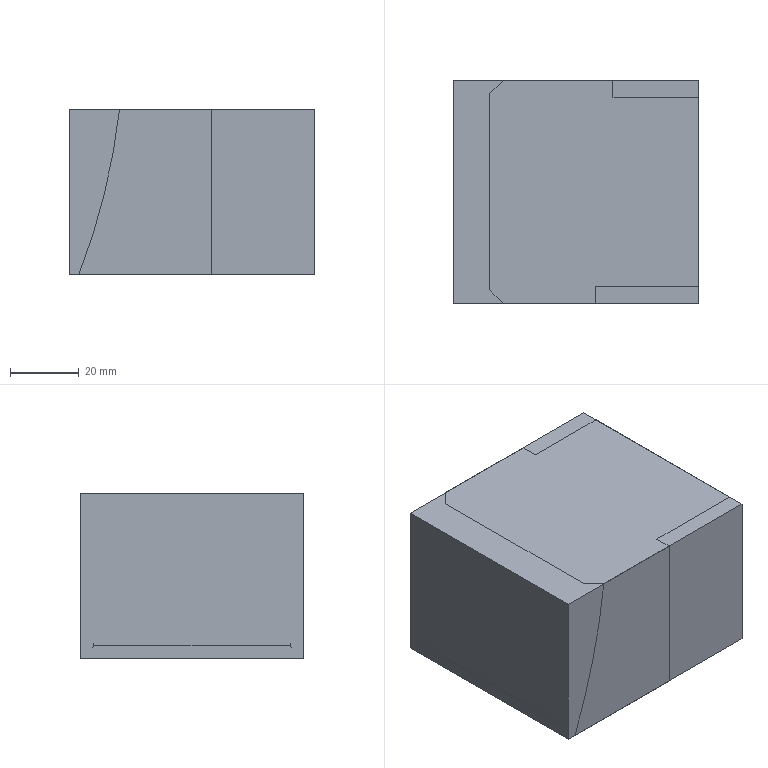NC program | NX | posted with a generic post | part box 71.51 x 65 x 48 mm
Lines 3301 to 3379 of 3379:
(ZLEVEL_PROFILE_COPY_COPY_COPY , TOOL : D10JING)
N6594 T11 M6
N6596 G54
N6598 G17 G0 G90 X-42.565 Y-34.122 B0. C0. S9500 M3
N6600 G43 Z30. H11
N6602 Z-13.
N6604 G94 G1 Z-16. F1000.
N6606 X-41.255 Y-33.366
N6608 G3 X-40.755 Y-32.5 R1.
N6610 G1 Y32.5 F1500.
N6612 G2 X-35.755 Y37.5 R5.
N6614 G1 X35.755
N6616 G2 X40.755 Y32.5 R5.
N6618 G1 Y-32.5
N6620 G2 X35.755 Y-37.5 R5.
N6622 G1 X-35.755
N6624 G2 X-40.755 Y-32.5 R5.
N6626 G3 X-41.255 Y-31.634 R1.
N6628 G1 X-42.755 Y-30.768
N6630 Z-13.
N6632 G0 X-42.565 Y-34.122 Z-29.
N6634 G1 Z-32. F1000.
N6636 X-41.255 Y-33.366
N6638 G3 X-40.755 Y-32.5 R1.
N6640 G1 Y32.5 F1500.
N6642 G2 X-35.755 Y37.5 R5.
N6644 G1 X35.755
N6646 G2 X40.755 Y32.5 R5.
N6648 G1 Y-32.5
N6650 G2 X35.755 Y-37.5 R5.
N6652 G1 X-35.755
N6654 G2 X-40.755 Y-32.5 R5.
N6656 G3 X-41.255 Y-31.634 R1.
N6658 G1 X-42.755 Y-30.768
N6660 Z-29.
N6662 G0 X-42.565 Y-34.122 Z-45.
N6664 G1 Z-48. F1000.
N6666 X-41.255 Y-33.366
N6668 G3 X-40.755 Y-32.5 R1.
N6670 G1 Y32.5 F1500.
N6672 G2 X-35.755 Y37.5 R5.
N6674 G1 X35.755
N6676 G2 X40.755 Y32.5 R5.
N6678 G1 Y-32.5
N6680 G2 X35.755 Y-37.5 R5.
N6682 G1 X-35.755
N6684 G2 X-40.755 Y-32.5 R5.
N6686 G3 X-41.255 Y-31.634 R1.
N6688 G1 X-42.755 Y-30.768
N6690 Z-45.
N6692 G0 Z30.
N6694 M5
(ZLEVEL_PROFILE_1_COPY_1 , TOOL : D6A45)
N6696 T07 M6
N6698 G54
N6700 G17 G0 G90 X-36.676 Y34.453 B0. C0. S9500 M3
N6702 G43 Z30. H7
N6704 Z0.
N6706 G94 G1 Z-1. F1000.
N6708 X-36.275 Y33.759
N6710 G3 X-35.756 Y33.459 R0.6
N6712 G1 X35.756
N6714 G2 X36.714 Y32.501 R0.958
N6716 G1 Y-32.501
N6718 G2 X35.756 Y-33.459 R0.958
N6720 G1 X-35.756
N6722 G2 X-36.714 Y-32.501 R0.958
N6724 G1 Y32.501
N6726 G2 X-35.756 Y33.459 R0.958
N6728 G3 X-35.236 Y33.759 R0.6
N6730 G1 X-34.717 Y34.659
N6732 Z0.
N6734 G0 Z30.
N6736 M5
N6738 M2